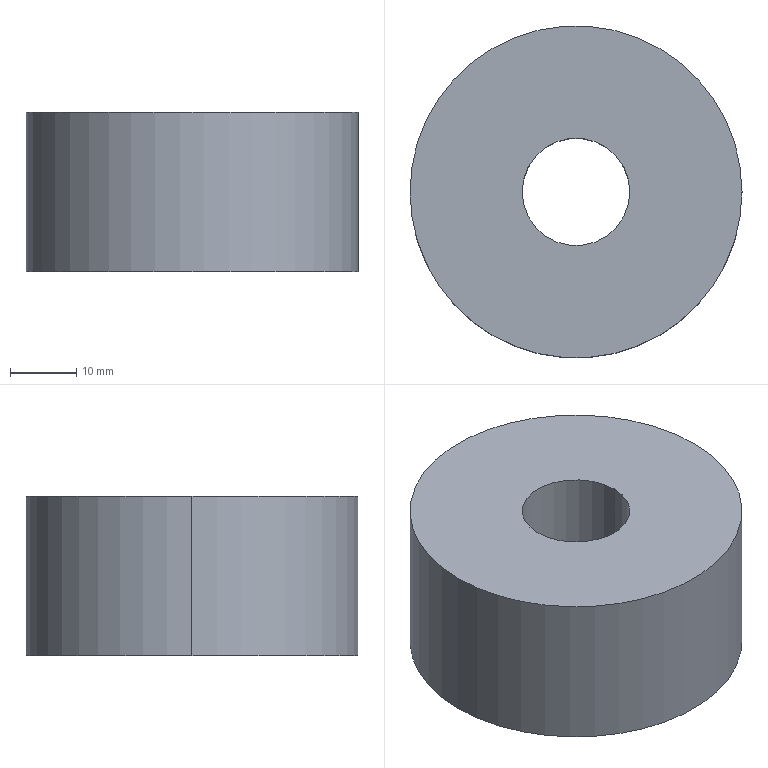Part | SolidWorks | features Extrusion 1 | 1 solid | 6 faces | box 50 x 50 x 24 mm | volume 42177 mm3 | cylinder 4 | plane 2 | commonest cylinder face diameters 16.2 x2 50 x2
STEP:
#1=CARTESIAN_POINT('',(-8.1,0.,-12.));
#2=VERTEX_POINT('',#1);
#3=CARTESIAN_POINT('',(8.1,0.,-12.));
#4=VERTEX_POINT('',#3);
#5=CARTESIAN_POINT('',(0.,0.,-12.));
#6=DIRECTION('',(0.,0.,1.));
#7=DIRECTION('',(1.,0.,0.));
#8=AXIS2_PLACEMENT_3D('',#5,#6,#7);
#9=CIRCLE('',#8,8.1);
#10=EDGE_CURVE('',#2,#4,#9,.T.);
#11=ORIENTED_EDGE('',*,*,#10,.F.);
#12=CARTESIAN_POINT('',(-8.1,0.,12.));
#13=VERTEX_POINT('',#12);
#14=CARTESIAN_POINT('',(-8.1,0.,-12.));
#15=DIRECTION('',(0.,0.,1.));
#16=VECTOR('',#15,1000.);
#17=LINE('',#14,#16);
#18=EDGE_CURVE('',#2,#13,#17,.T.);
#19=ORIENTED_EDGE('',*,*,#18,.T.);
#20=CARTESIAN_POINT('',(8.1,0.,12.));
#21=VERTEX_POINT('',#20);
#22=CARTESIAN_POINT('',(0.,0.,12.));
#23=DIRECTION('',(0.,0.,1.));
#24=DIRECTION('',(1.,0.,0.));
#25=AXIS2_PLACEMENT_3D('',#22,#23,#24);
#26=CIRCLE('',#25,8.1);
#27=EDGE_CURVE('',#13,#21,#26,.T.);
#28=ORIENTED_EDGE('',*,*,#27,.T.);
#29=CARTESIAN_POINT('',(8.1,0.,-12.));
#30=DIRECTION('',(0.,0.,1.));
#31=VECTOR('',#30,1000.);
#32=LINE('',#29,#31);
#33=EDGE_CURVE('',#4,#21,#32,.T.);
#34=ORIENTED_EDGE('',*,*,#33,.F.);
#35=EDGE_LOOP('',(#11,#19,#28,#34));
#36=FACE_OUTER_BOUND('',#35,.T.);
#37=CARTESIAN_POINT('',(0.,0.,-12.));
#38=DIRECTION('',(0.,0.,1.));
#39=DIRECTION('',(1.,0.,0.));
#40=AXIS2_PLACEMENT_3D('',#37,#38,#39);
#41=CYLINDRICAL_SURFACE('',#40,8.1);
#42=ADVANCED_FACE('',(#36),#41,.F.);
#43=CARTESIAN_POINT('',(25.,0.,-12.));
#44=VERTEX_POINT('',#43);
#45=CARTESIAN_POINT('',(-25.,0.,-12.));
#46=VERTEX_POINT('',#45);
#47=CARTESIAN_POINT('',(0.,0.,-12.));
#48=DIRECTION('',(0.,0.,1.));
#49=DIRECTION('',(1.,0.,0.));
#50=AXIS2_PLACEMENT_3D('',#47,#48,#49);
#51=CIRCLE('',#50,25.);
#52=EDGE_CURVE('',#44,#46,#51,.T.);
#53=ORIENTED_EDGE('',*,*,#52,.T.);
#54=CARTESIAN_POINT('',(-25.,0.,12.));
#55=VERTEX_POINT('',#54);
#56=CARTESIAN_POINT('',(-25.,0.,-12.));
#57=DIRECTION('',(0.,0.,1.));
#58=VECTOR('',#57,1000.);
#59=LINE('',#56,#58);
#60=EDGE_CURVE('',#46,#55,#59,.T.);
#61=ORIENTED_EDGE('',*,*,#60,.T.);
#62=CARTESIAN_POINT('',(25.,0.,12.));
#63=VERTEX_POINT('',#62);
#64=CARTESIAN_POINT('',(0.,0.,12.));
#65=DIRECTION('',(0.,0.,1.));
#66=DIRECTION('',(1.,0.,0.));
#67=AXIS2_PLACEMENT_3D('',#64,#65,#66);
#68=CIRCLE('',#67,25.);
#69=EDGE_CURVE('',#63,#55,#68,.T.);
#70=ORIENTED_EDGE('',*,*,#69,.F.);
#71=CARTESIAN_POINT('',(25.,0.,-12.));
#72=DIRECTION('',(0.,0.,1.));
#73=VECTOR('',#72,1000.);
#74=LINE('',#71,#73);
#75=EDGE_CURVE('',#44,#63,#74,.T.);
#76=ORIENTED_EDGE('',*,*,#75,.F.);
#77=EDGE_LOOP('',(#53,#61,#70,#76));
#78=FACE_OUTER_BOUND('',#77,.T.);
#79=CARTESIAN_POINT('',(0.,0.,-12.));
#80=DIRECTION('',(0.,0.,1.));
#81=DIRECTION('',(1.,0.,0.));
#82=AXIS2_PLACEMENT_3D('',#79,#80,#81);
#83=CYLINDRICAL_SURFACE('',#82,25.);
#84=ADVANCED_FACE('',(#78),#83,.T.);
#85=ORIENTED_EDGE('',*,*,#60,.F.);
#86=CARTESIAN_POINT('',(0.,0.,-12.));
#87=DIRECTION('',(0.,0.,1.));
#88=DIRECTION('',(1.,0.,0.));
#89=AXIS2_PLACEMENT_3D('',#86,#87,#88);
#90=CIRCLE('',#89,25.);
#91=EDGE_CURVE('',#46,#44,#90,.T.);
#92=ORIENTED_EDGE('',*,*,#91,.T.);
#93=ORIENTED_EDGE('',*,*,#75,.T.);
#94=CARTESIAN_POINT('',(0.,0.,12.));
#95=DIRECTION('',(0.,0.,1.));
#96=DIRECTION('',(1.,0.,0.));
#97=AXIS2_PLACEMENT_3D('',#94,#95,#96);
#98=CIRCLE('',#97,25.);
#99=EDGE_CURVE('',#55,#63,#98,.T.);
#100=ORIENTED_EDGE('',*,*,#99,.F.);
#101=EDGE_LOOP('',(#85,#92,#93,#100));
#102=FACE_OUTER_BOUND('',#101,.T.);
#103=CARTESIAN_POINT('',(0.,0.,-12.));
#104=DIRECTION('',(0.,0.,1.));
#105=DIRECTION('',(1.,0.,0.));
#106=AXIS2_PLACEMENT_3D('',#103,#104,#105);
#107=CYLINDRICAL_SURFACE('',#106,25.);
#108=ADVANCED_FACE('',(#102),#107,.T.);
#109=CARTESIAN_POINT('',(0.,0.,-12.));
#110=DIRECTION('',(0.,0.,1.));
#111=DIRECTION('',(1.,0.,0.));
#112=AXIS2_PLACEMENT_3D('',#109,#110,#111);
#113=CIRCLE('',#112,8.1);
#114=EDGE_CURVE('',#4,#2,#113,.T.);
#115=ORIENTED_EDGE('',*,*,#114,.T.);
#116=ORIENTED_EDGE('',*,*,#10,.T.);
#117=EDGE_LOOP('',(#115,#116));
#118=FACE_BOUND('',#117,.T.);
#119=ORIENTED_EDGE('',*,*,#52,.F.);
#120=ORIENTED_EDGE('',*,*,#91,.F.);
#121=EDGE_LOOP('',(#119,#120));
#122=FACE_OUTER_BOUND('',#121,.T.);
#123=CARTESIAN_POINT('',(0.,0.,-12.));
#124=DIRECTION('',(0.,0.,1.));
#125=DIRECTION('',(1.,0.,0.));
#126=AXIS2_PLACEMENT_3D('',#123,#124,#125);
#127=PLANE('',#126);
#128=ADVANCED_FACE('',(#118,#122),#127,.F.);
#129=CARTESIAN_POINT('',(0.,0.,12.));
#130=DIRECTION('',(0.,0.,1.));
#131=DIRECTION('',(1.,0.,0.));
#132=AXIS2_PLACEMENT_3D('',#129,#130,#131);
#133=CIRCLE('',#132,8.1);
#134=EDGE_CURVE('',#21,#13,#133,.T.);
#135=ORIENTED_EDGE('',*,*,#134,.F.);
#136=ORIENTED_EDGE('',*,*,#27,.F.);
#137=EDGE_LOOP('',(#135,#136));
#138=FACE_BOUND('',#137,.T.);
#139=ORIENTED_EDGE('',*,*,#69,.T.);
#140=ORIENTED_EDGE('',*,*,#99,.T.);
#141=EDGE_LOOP('',(#139,#140));
#142=FACE_OUTER_BOUND('',#141,.T.);
#143=CARTESIAN_POINT('',(0.,0.,12.));
#144=DIRECTION('',(0.,0.,1.));
#145=DIRECTION('',(1.,0.,0.));
#146=AXIS2_PLACEMENT_3D('',#143,#144,#145);
#147=PLANE('',#146);
#148=ADVANCED_FACE('',(#138,#142),#147,.T.);
#149=ORIENTED_EDGE('',*,*,#18,.F.);
#150=ORIENTED_EDGE('',*,*,#114,.F.);
#151=ORIENTED_EDGE('',*,*,#33,.T.);
#152=ORIENTED_EDGE('',*,*,#134,.T.);
#153=EDGE_LOOP('',(#149,#150,#151,#152));
#154=FACE_OUTER_BOUND('',#153,.T.);
#155=CARTESIAN_POINT('',(0.,0.,-12.));
#156=DIRECTION('',(0.,0.,1.));
#157=DIRECTION('',(1.,0.,0.));
#158=AXIS2_PLACEMENT_3D('',#155,#156,#157);
#159=CYLINDRICAL_SURFACE('',#158,8.1);
#160=ADVANCED_FACE('',(#154),#159,.F.);
#161=CLOSED_SHELL('',(#42,#84,#108,#128,#148,#160));
#162=MANIFOLD_SOLID_BREP('',#161);
#163=CARTESIAN_POINT('',(0.,0.,0.));
#164=DIRECTION('',(0.,0.,1.));
#165=DIRECTION('',(1.,0.,0.));
#166=AXIS2_PLACEMENT_3D('',#163,#164,#165);
#167=(LENGTH_UNIT()NAMED_UNIT(*)SI_UNIT(.MILLI.,.METRE.));
#168=UNCERTAINTY_MEASURE_WITH_UNIT(LENGTH_MEASURE(0.00001),#167,'','');
#169=(NAMED_UNIT(*)PLANE_ANGLE_UNIT()SI_UNIT($,.RADIAN.));
#170=(NAMED_UNIT(*)SI_UNIT($,.STERADIAN.)SOLID_ANGLE_UNIT());
#171=(GEOMETRIC_REPRESENTATION_CONTEXT(3)GLOBAL_UNCERTAINTY_ASSIGNED_CONTEXT((#168))GLOBAL_UNIT_ASSIGNED_CONTEXT((#167,#169,#170))REPRESENTATION_CONTEXT('',''));
#172=ADVANCED_BREP_SHAPE_REPRESENTATION('',(#162,#166),#171);